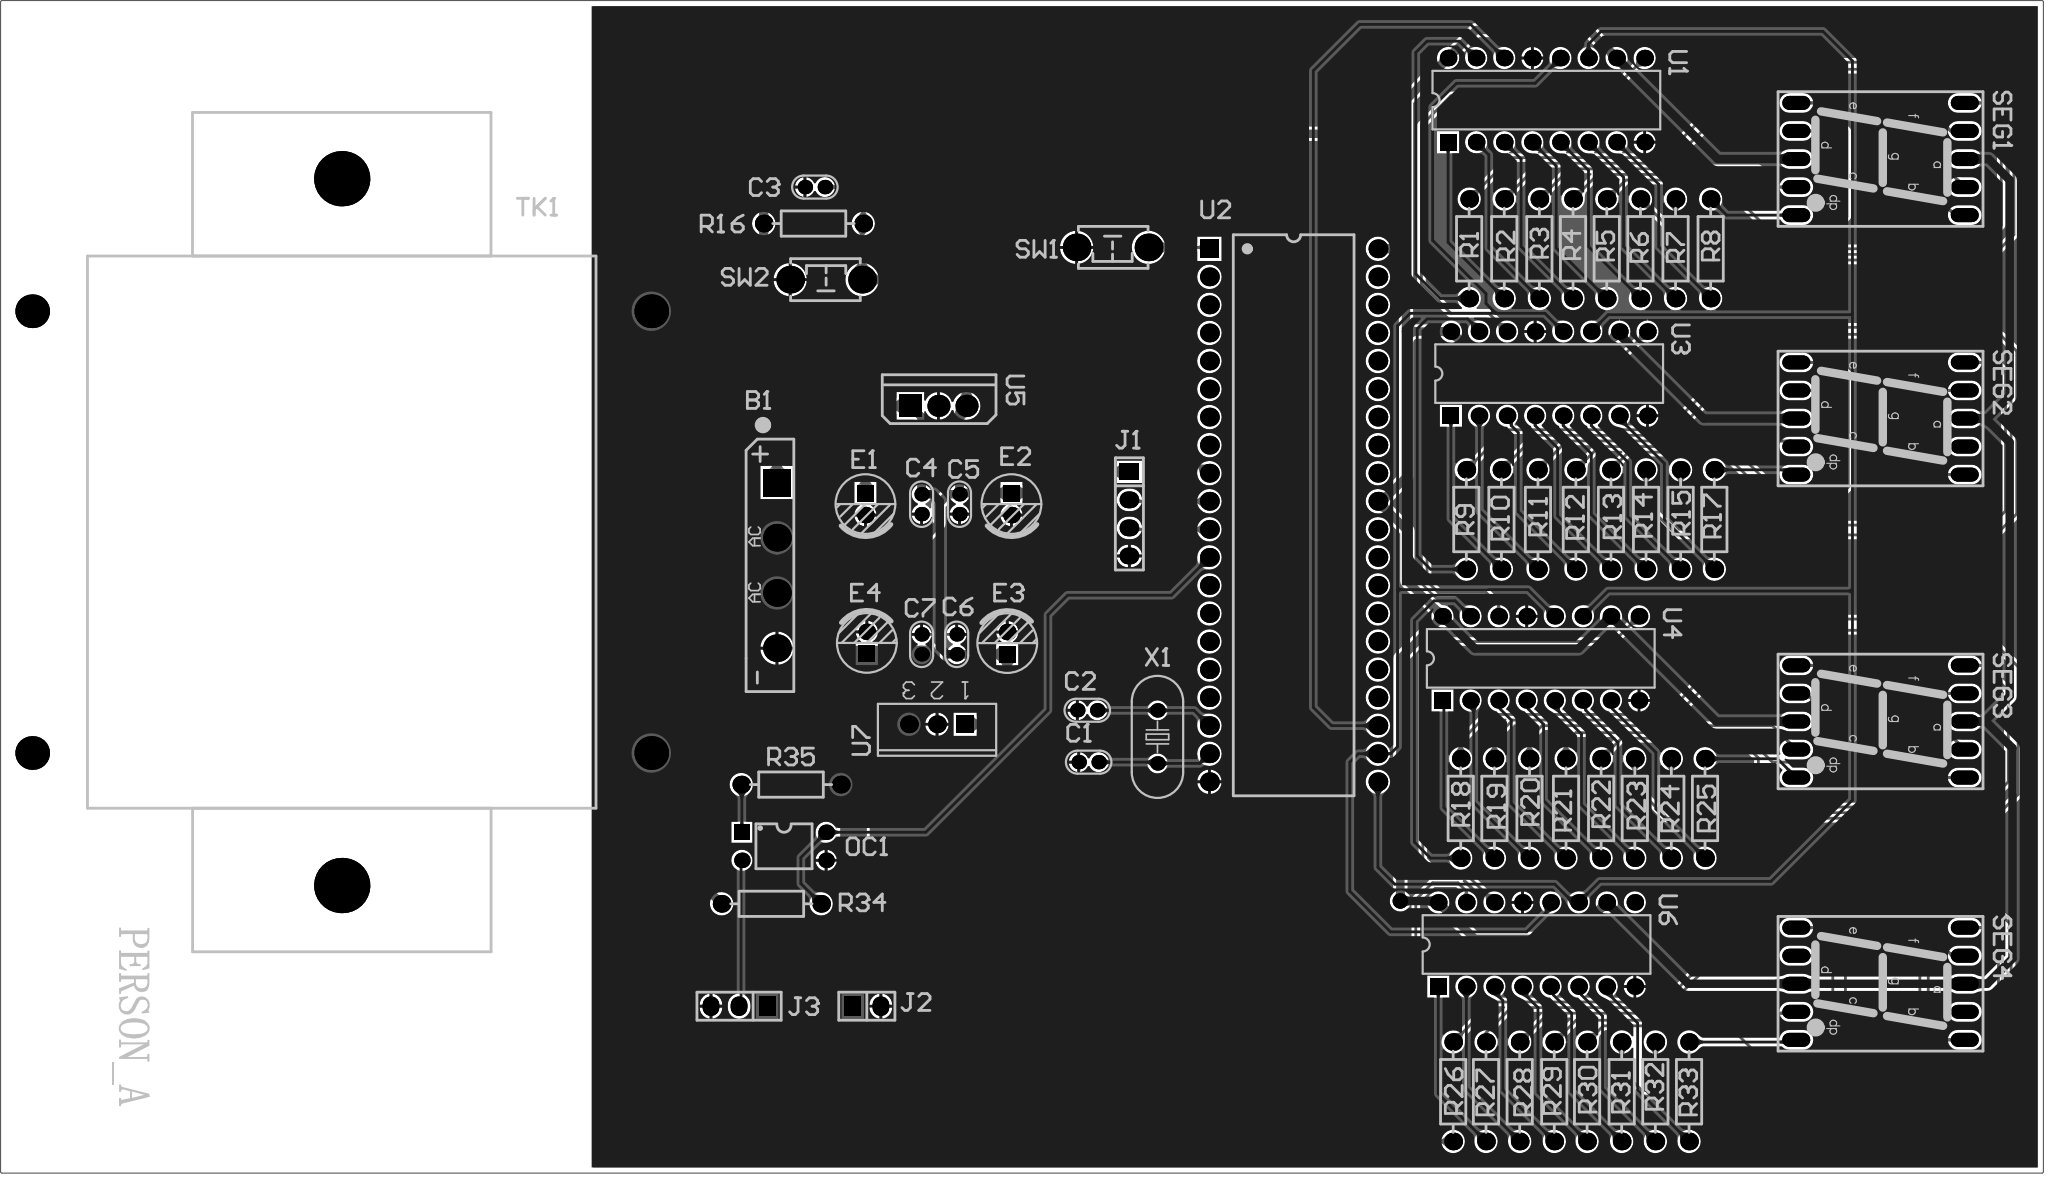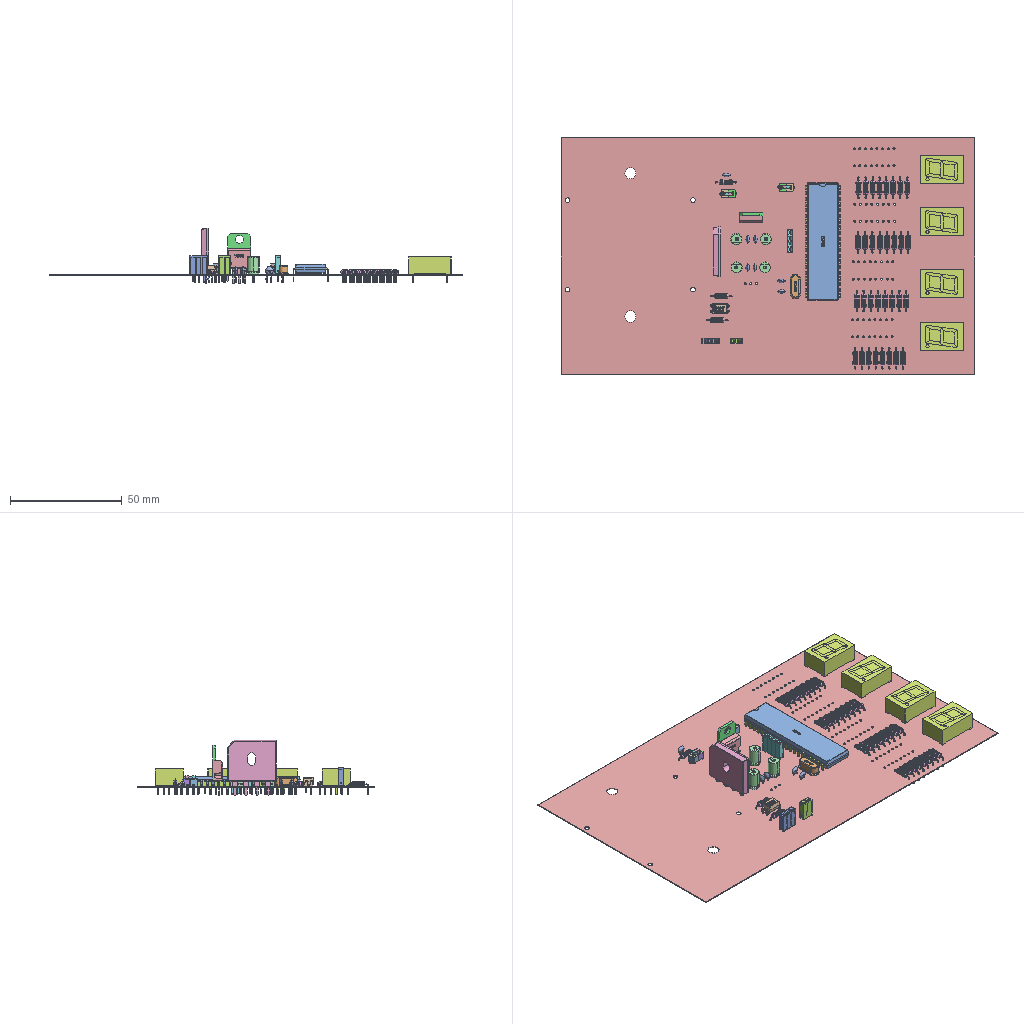Circuit board layout | Altium Designer | box 184.8 x 106.2 x 24.8 mm
Layer stack:
# Altium Designer layer stack of  (unit mm; dielectric type: 0 none, 1 core, 2 prepreg, 3 surface material)
index,name,kind,layer,copper_thickness_mm,dielectric_type,dielectric_thickness_mm,dielectric_material,dielectric_constant
0,Top Paste,other,,,,,,
1,Top Overlay,other,,,,,,
2,Top Solder,dielectric,,,3,0.0102,Solder Resist,3.5
3,Top Layer,copper,Top Layer,0.0356,,,,
4,Dielectric 1,dielectric,,,0,0.32,FR-4,4.8
5,Bottom Layer,copper,Bottom Layer,0.0356,,,,
6,Bottom Solder,dielectric,,,3,0.0102,Solder Resist,3.5
7,Bottom Overlay,other,,,,,,
8,Bottom Paste,other,,,,,,
# drill layer pairs: low layer,high layer
drill_pair,Top Layer,Bottom Layer
Part placement:
Designator,Comment,Layer,Footprint,Center-X(mm),Center-Y(mm),Rotation
J3,Female HDR1X3,TopLayer,Fe-HDR1X3/2.54-S,91.186,40.386,270
J2,Female HDR1X2,TopLayer,Fe-HDR1X2/2.54-S,102.743,40.386,360
X1,12MHz,TopLayer,OSC_HC-49S,129.032,64.77,270
U7,LM7812CT,TopLayer,T03B,109.093,65.913,180
U6,SN74LS595,TopLayer,DIP-16,163.322,45.974,360
U5,LM7805,TopLayer,TO220A,109.22,94.742,360
U4,SN74LS595,TopLayer,DIP-16,163.703,71.882,360
U3,SN74LS595,TopLayer,DIP-16,164.465,97.663,360
U2,AT89C51,TopLayer,DIP40,141.351,84.836,360
U1,SN74LS595,TopLayer,DIP-16,164.211,122.428,360
TK1,TRAN-2P2S,TopLayer,TRANS2P2S,55.245,83.312,90
SW1,3x6x5,TopLayer,TSW_DIP-3*6*5,124.968,109.093,180
SEG4,0.56IN-1-A,TopLayer,0.56IN-1P,194.437,42.418,270
SEG3,0.56IN-1-A,TopLayer,0.56IN-1P,194.437,66.167,270
SEG2,0.56IN-1-A,TopLayer,0.56IN-1P,194.437,93.599,270
SEG1,0.56IN-1-A,TopLayer,0.56IN-1P,194.437,117.094,270
R35,1K,TopLayer,RS_1/4W,95.885,60.452,360
R34,10K,TopLayer,RS_1/4W,94.107,49.657,180
R33,100R,TopLayer,RS_1/4W,177.117,32.639,90
R32,100R,TopLayer,RS_1/4W,174.069,32.639,90
R31,100R,TopLayer,RS_1/4W,171.021,32.639,90
R30,100R,TopLayer,RS_1/4W,167.894,32.639,90
R29,100R,TopLayer,RS_1/4W,164.925,32.639,90
R28,100R,TopLayer,RS_1/4W,161.798,32.639,90
R27,100R,TopLayer,RS_1/4W,158.75,32.639,90
R26,100R,TopLayer,RS_1/4W,155.781,32.639,90
R25,100R,TopLayer,RS_1/4W,178.562,58.293,90
R24,100R,TopLayer,RS_1/4W,175.514,58.293,90
R23,100R,TopLayer,RS_1/4W,172.212,58.293,90
R22,100R,TopLayer,RS_1/4W,169.164,58.293,90
R21,100R,TopLayer,RS_1/4W,165.989,58.293,90
R20,100R,TopLayer,RS_1/4W,162.687,58.293,90
R19,100R,TopLayer,RS_1/4W,159.512,58.293,90
R18,100R,TopLayer,RS_1/4W,156.464,58.293,90
R17,100R,TopLayer,RS_1/4W,179.403,84.455,90
R15,100R,TopLayer,RS_1/4W,176.355,84.455,90
R14,100R,TopLayer,RS_1/4W,173.228,84.455,90
R13,100R,TopLayer,RS_1/4W,170.053,84.455,90
R12,100R,TopLayer,RS_1/4W,166.878,84.455,90
R11,100R,TopLayer,RS_1/4W,163.449,84.455,90
R10,100R,TopLayer,RS_1/4W,160.147,84.455,90
R9,100R,TopLayer,RS_1/4W,156.972,84.455,90
R8,100R,TopLayer,RS_1/4W,179.07,108.966,90
R7,100R,TopLayer,RS_1/4W,175.895,108.966,90
R6,100R,TopLayer,RS_1/4W,172.72,108.966,90
R5,100R,TopLayer,RS_1/4W,169.672,108.966,90
R4,100R,TopLayer,RS_1/4W,166.624,108.966,90
R3,100R,TopLayer,RS_1/4W,163.576,108.966,90
R2,100R,TopLayer,RS_1/4W,160.401,108.966,90
R1,100R,TopLayer,RS_1/4W,157.226,108.966,90
OC1,PC817,TopLayer,DIP_PC817,95.25,54.864,360
E4,220U,TopLayer,CS_2.0*5*8_-_C,102.743,73.279,270
E3,220U,TopLayer,CS_2.0*5*8_-_C,115.443,73.263,270
E2,220U,TopLayer,CS_2.0*5*8_-_C,115.824,85.852,90
E1,220U,TopLayer,CS_2.0*5*8_-_C,102.616,85.852,90
C7,1nF,TopLayer,CC_1.8*3.6,107.696,73.152,270
C6,1nF,TopLayer,CC_1.8*3.6,110.871,73.152,270
C5,1nF,TopLayer,CC_1.8*3.6,111.125,85.841,90
C4,1nF,TopLayer,CC_1.8*3.6,107.696,85.841,90
C2,1nF,TopLayer,CC_1.8*3.6,122.682,67.183,0
C1,1nF,TopLayer,CC_1.8*3.6,122.809,62.484,0
B1,GBU,TopLayer,GBU,94.615,80.304,90
C3,100nF,TopLayer,CC_1.8*3.6,98.044,114.554,360
R16,10K,TopLayer,RS_1/4W,97.917,111.252,180
SW2,3x6x5,TopLayer,TSW_DIP-3*6*5,99.06,106.172,360
J1,Female HDR1X4,TopLayer,Fe-HDR1X4/2.54-S,126.492,84.963,0
Pad and via stacks:
# Altium Designer via and pad stacks of  (unit mm). Each distinct definition once, with the count of objects using it.
# via: kind,start_layer,end_layer,hole_mm,diameter_mm,mode(0 simple;1 top-mid-bottom;2 full stack),diameter_per_layer,count,example_net
# pad: kind,layer,hole_mm,hole_type(0 round;1 square;2 slot),plating,top_size,top_shape(1 round;2 rect;3 octagon;9 rounded rect),mid_size,bottom_size,mode,footprint,size_per_layer,count,example
pad,Multi-Layer,0.8128,0,plated,1.524x1.778,2,1.524x1.778,1.524x1.778,0,Fe-HDR1X3/2.54-S,,1,J3.1
pad,Multi-Layer,0.8128,0,plated,1.524x1.778,1,1.524x1.778,1.524x1.778,0,Fe-HDR1X3/2.54-S,,2,J3.2
pad,Multi-Layer,0.8128,0,plated,1.524x1.778,2,1.524x1.778,1.524x1.778,0,Fe-HDR1X2/2.54-S,,1,J2.1
pad,Multi-Layer,0.8128,0,plated,1.524x1.778,1,1.524x1.778,1.524x1.778,0,Fe-HDR1X2/2.54-S,,1,J2.2
pad,Multi-Layer,0.9,0,plated,1.5x1.5,1,1.5x1.5,1.5x1.5,0,DIP-16,,60,U1.9
pad,Multi-Layer,0.9,0,plated,1.5x1.5,2,1.5x1.5,1.5x1.5,0,DIP-16,,4,U1.1
pad,Multi-Layer,0.6,0,plated,1.6x1.6,1,1.6x1.6,1.6x1.6,0,RS 1/4W,,70,R1.2
pad,Multi-Layer,0.8,0,plated,1.7x1.7,1,1.7x1.7,1.7x1.7,0,DIP40,,39,U2.21
pad,Multi-Layer,0.8,0,plated,1.7x1.7,2,1.7x1.7,1.7x1.7,0,DIP40,,1,U2.1
pad,Multi-Layer,1.2,0,plated,2.5x2.5,1,2.5x2.5,2.5x2.5,0,TSW DIP-3*6*5,,4,SW1.1
pad,Multi-Layer,0.85,0,plated,2.54x1.27,1,2.54x1.27,2.54x1.27,0,0.56IN-1P,,40,SEG1.10
pad,Multi-Layer,0.5,0,plated,1.3x1.3,1,1.3x1.3,1.3x1.3,0,CC 1.8*3.6,,14,C1.2
pad,Multi-Layer,0.6,0,plated,1.3x1.3,1,1.3x1.3,1.3x1.3,0,OSC HC-49S,,2,X1.2
pad,Multi-Layer,2.032,0,plated,3.048x3.048,1,3.048x3.048,3.048x3.048,0,TRANS2P2S,,4,TK1.3
pad,Multi-Layer,5,0,unplated,5x5,1,5x5,5x5,0,TRANS2P2S,,2,TK1.
pad,Multi-Layer,1.5,0,plated,2.5x2.5,2,2.5x2.5,2.5x2.5,0,GBU,,1,B1.DC+
pad,Multi-Layer,1.5,0,plated,2.5x2.5,1,2.5x2.5,2.5x2.5,0,GBU,,3,B1.AC2
pad,Multi-Layer,0.8,0,plated,1.5x1.5,2,1.5x1.5,1.5x1.5,0,CS 2.0*5*8 - C,,4,E2.1
pad,Multi-Layer,0.8,0,plated,1.5x1.5,1,1.5x1.5,1.5x1.5,0,CS 2.0*5*8 - C,,4,E2.2
pad,Multi-Layer,0.8128,0,plated,1.4x1.4,2,1.4x1.4,1.4x1.4,0,DIP_PC817,,1,OC1.1
pad,Multi-Layer,0.8128,0,plated,1.4x1.4,1,1.4x1.4,1.4x1.4,0,DIP_PC817,,3,OC1.2
pad,Multi-Layer,1.1,0,plated,2x2,2,2x2,2x2,0,TO220A,,1,U5.1
pad,Multi-Layer,1.1,0,plated,2x2,1,2x2,2x2,0,TO220A,,2,U5.3
pad,Multi-Layer,1,0,plated,1.6x1.6,1,1.6x1.6,1.6x1.6,0,T03B,,2,U7.3
pad,Multi-Layer,1,0,plated,1.6x1.6,2,1.6x1.6,1.6x1.6,0,T03B,,1,U7.1
pad,Multi-Layer,0.8128,0,plated,1.524x1.778,2,1.524x1.778,1.524x1.778,0,Fe-HDR1X4/2.54-S,,1,J1.1
pad,Multi-Layer,0.8128,0,plated,1.524x1.778,1,1.524x1.778,1.524x1.778,0,Fe-HDR1X4/2.54-S,,3,J1.2
via,Top Layer,Bottom Layer,0.8,1.4,0,,1,VCC
Copper pours:
name,layer,net,type(0 solid;1 hatched;2 none)
D,Top Layer,GND,0
D,Bottom Layer,GND,0
Design rules, without the lines most boards share:
# Altium Designer design rules of  (exported by Altium Designer, unit mm)
# columns: name | kind | enabled | priority | scope1 | scope2 | descriptor | typed fields (field=value)
Clearance | 0 | enabled | 1 | All | All | Clearance Constraint (Gap=10mil) (All),(All) | gap=0.254
PlaneConnect | 6 | enabled | 1 | All | All | Power Plane Connect Rule(Relief Connect )(Expansion=20mil) (Conductor Width=10mil) (Air Gap=10mil) (Entries=4) (All) | relief_conductor_width=0.254 relief_entries=4 relief_expansion=0.508
PolygonConnect | 20 | enabled | 1 | All | All | Polygon Connect Rule(Relief Connect )(Conductor Width=10mil) (Relief Angle=90 Angle) (Entries=4) (Air Gap Width=10mil) (All),(All) | connect_style(0=relief,1=direct,2=none)=0 relief_conductor_width=0.254 relief_entries=4
Width | 2 | enabled | 1 | All | All | Width Constraint (Min=10mil) (Max=60mil) (Preferred=10mil) (All) |
RoutingVias | 11 | enabled | 1 | All | All | Routing Via (MinHoleWidth=28mil) (MaxHoleWidth=28mil) (PreferredHoleWidth=28mil) (MinWidth=50mil) (MaxWidth=50mil) (PreferedWidth=50mil) (All) | via_min_hole=0.7112 via_max_hole=0.7112 via_preferred_diameter=1.27 via_preferred_hole=0.7112
PasteMaskExpansion | 14 | enabled | 1 | All | All | Paste Mask Expansion (Expansion =0mil) (All) | expansion=0
SolderMaskExpansion | 13 | enabled | 1 | All | All | Solder Mask Expansion (Expansion =4mil) (All) | expansion=0.1016
HoleSize | 42 | enabled | 1 | All | All | Hole Size Constraint (Min=1mil) (Max=1000mil) (All) |
DiffPairsRouting | 51 | enabled | 1 | All | All | Differential Pairs Uncoupled Length using the Gap Constraints (Min=10mil) (Max=10mil) (Prefered=10mil)  and Width Constraints (Min=15mil) (Max=15mil) (Prefered=15mil) (All) |
HoleToHoleClearance | 52 | enabled | 1 | All | All | Hole To Hole Clearance (Gap=10mil) (All),(All) | gap=0.254
MinimumSolderMaskSliver | 53 | enabled | 1 | All | All | Minimum Solder Mask Sliver (Gap=0mil) (All),(All) |
SilkToSolderMaskClearance | 54 | enabled | 1 | IsPad | All | Silk To Solder Mask (Clearance=0mil) (IsPad),(All) |
SilkToSilkClearance | 55 | enabled | 1 | All | All | Silk to Silk (Clearance=0mil) (All),(All) |
Classes set for this board:
# Altium Designer classes of  (member kind: 0 net, 1 component, 2 from-to, 3 pad, 4 layer, 5 differential pair, 6 design channel, 7 polygon, 8 structure, 9 xSignal)
# columns: class name | member kind | superclass | members
Sheet1 | 1 | no | B1; C1; C2; E1; E2; E3; E4; OC1; R1; R2; R3; R4; R5; R6; R7; R8; R9; R10; R11; R12; R13; R14; R15; SEG1; SEG2; SEG3; SEG4; SW1; TK1; U1; U2; U3; U4; U5; U6; U7; X1; C7; R35; SW2; R34; R22; R27; R18; R23; R30; R26; R33; C4; R21; R29; C7; R17; R25; R20; R32; C6; R28; R35; R19; R24; R31; C5; C3; J1; R16; J2; J3;